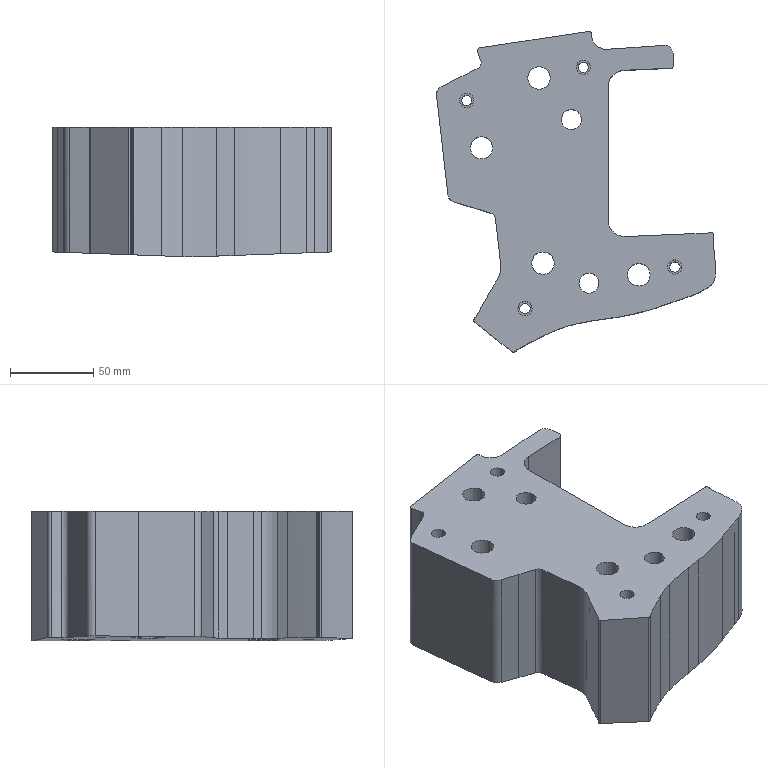Part | NX | features 8 2 | 1 solid | 88 faces | box 167.566 x 192.734 x 78 mm | volume 1280922 mm3 | cylinder 54 | plane 33 | spline 1 | commonest cylinder face diameters 2 x9 20 x6 6.2 x4 8.5 x4 13.5 x4 10 x3